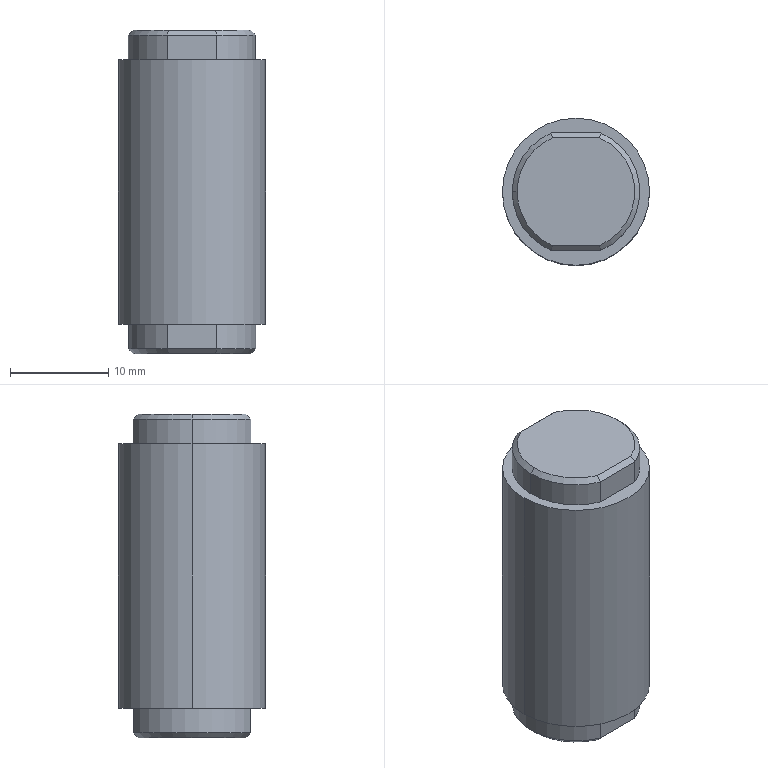Part | STEP file | Driven pulley support screw QY-1-35 | 1 solid | 26 faces | box 15 x 15 x 33 mm | volume 5538 mm3 | plane 12 | cylinder 8 | cone 6 | commonest cylinder face diameters 13 x6 15 x2